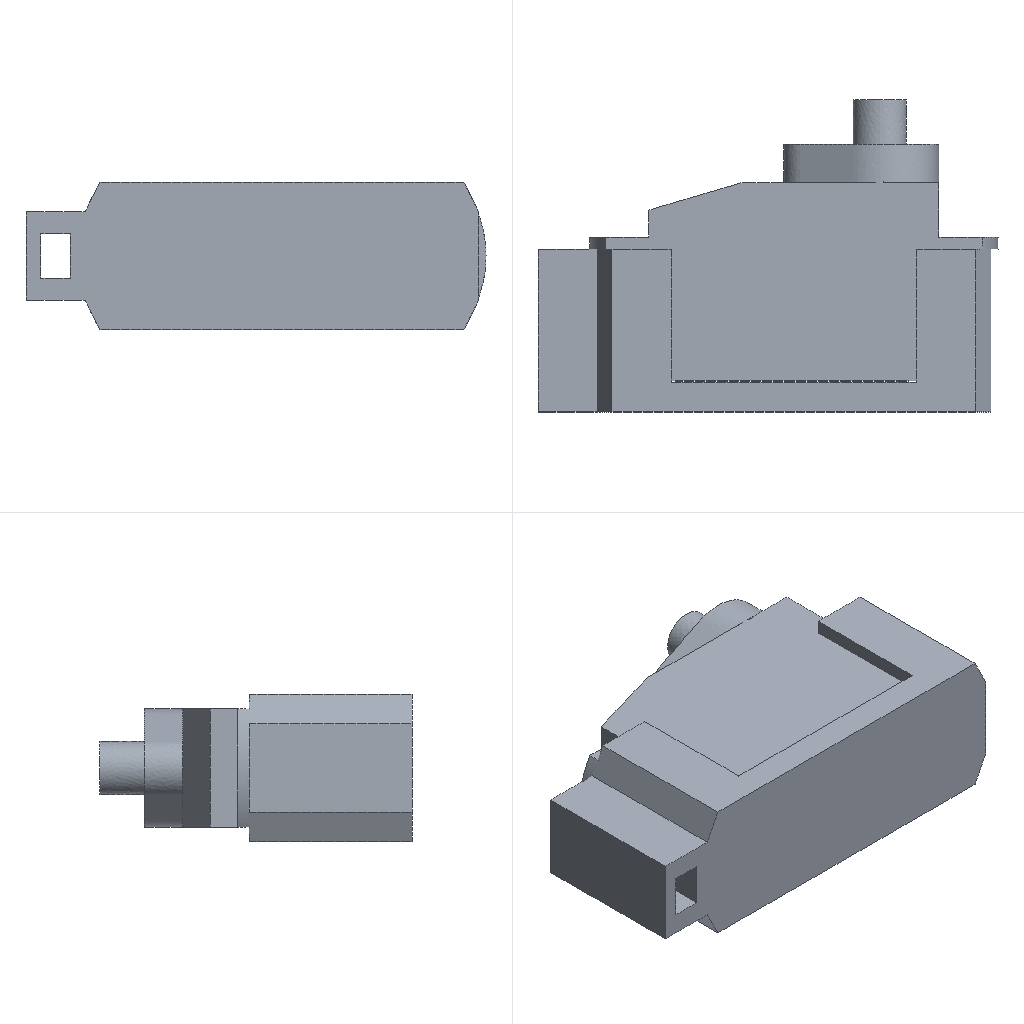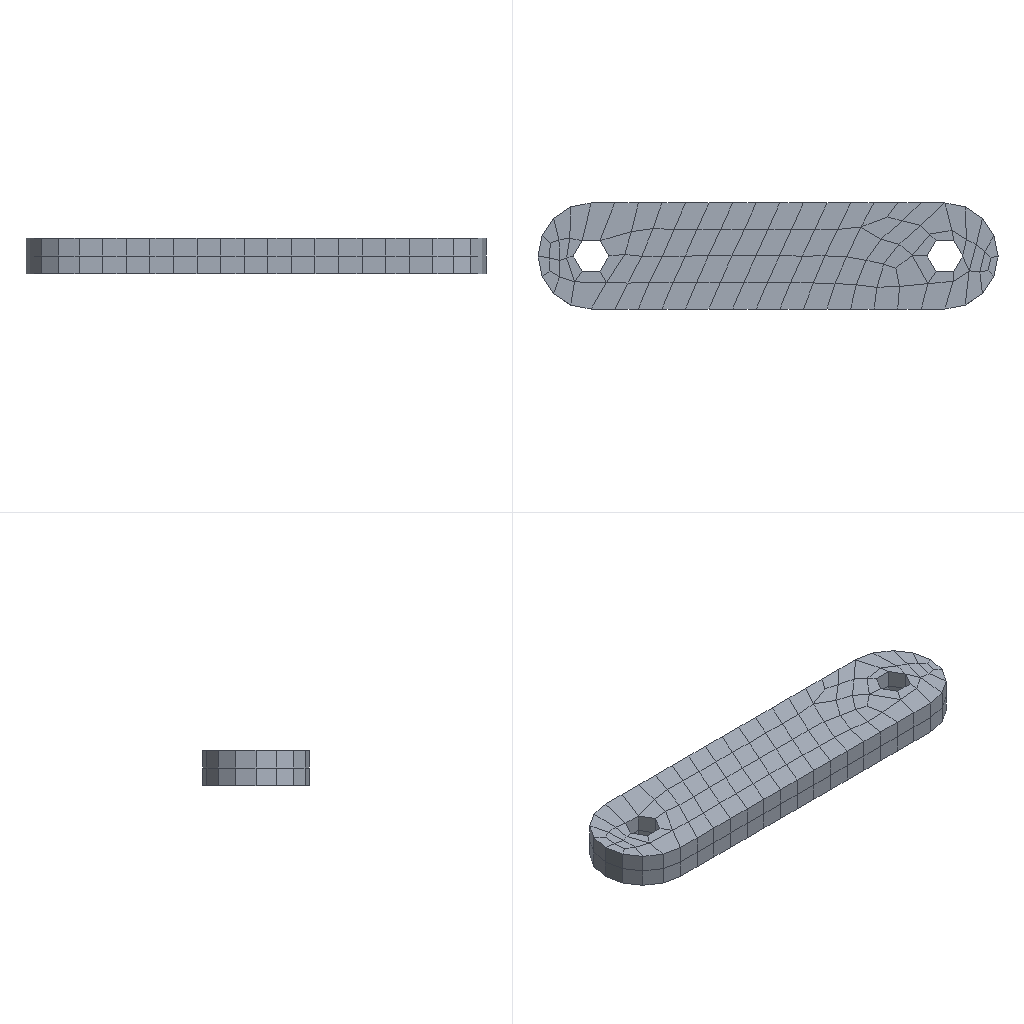Simulation study | ansys workbench
Set-up summary:
category,name,step,type,value,unit,region
solver,ansys_mapdl
solver,version,,,22.1
solver,version,,,22.1
units,MPA,,stated
analysis,deck1,,transient,transient
load_step,requested,,,1
analysis,nlgeom,,,True
mesh,nodes,,,1272
mesh,elements,,,190
element_type,ANSYS 186 (type 1),,solid,190
load,load commands in deck,,count,0
bc,support commands in deck,,count,1
named_set,_FIXEDSU,,component
analysis,deck2,,static,static
load_step,requested,,,1
analysis,nlgeom,,,False
mesh,nodes,,,104214
mesh,elements,,,70108
element_type,ANSYS 187 (type 1),,solid,30033
element_type,ANSYS 187 (type 2),,solid,29224
element_type,ANSYS 174 (type 3),,contact,4510
element_type,ANSYS 170 (type 4),,target,4510
element_type,ANSYS 154 (type 5),,surface,1333
element_type,ANSYS 154 (type 6),,surface,498
load,load commands in deck,,count,6
bc,support commands in deck,,count,1
named_set,_FIXEDSU,,component
material,1,,in results
material,1,,in results
material,2,,in results
check,setup vs results,,match
check,setup vs results,,match,1831 surface effect element(s) are not in the reader's mesh and were not compared
Results summary:
result,analysis,,,static
result,last_loadstep,,,1
result,primary field,,,displacement
result,reaction total,1,FX,-0.0,N
result,reaction total,1,FY,0.0,N
result,reaction total,1,FZ,-2e-06,N
result,mass,,,0.0,"NMM: mm, ton, N, s, mV, mA, degC"
result,analysis,,,static
result,last_loadstep,,,1
result,primary field,,,displacement
result,reaction total,1,FX,-0.0,N
result,reaction total,1,FY,-0.395,N
result,reaction total,1,FZ,-0.0,N
result,mass,,,5e-06,"NMM: mm, ton, N, s, mV, mA, degC"